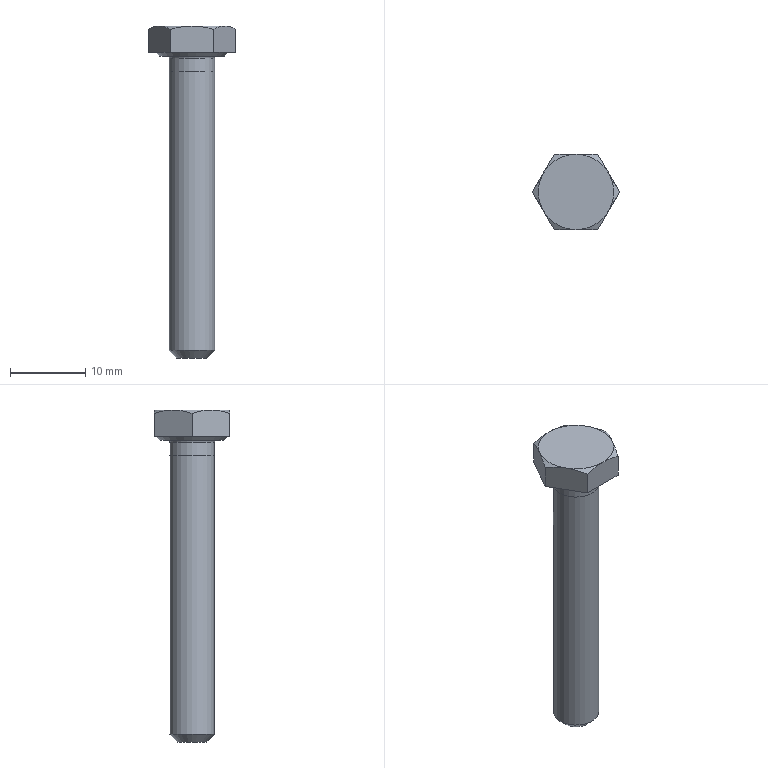Part | NX | features BREP 1, DATUM_CSYS 1 | 1 solid | 21 faces | box 11.547 x 10 x 44 mm | volume 1457 mm3 | plane 10 | cone 8 | cylinder 2 | torus 1 | commonest cylinder face diameters 6 x2
STEP:
#1=CARTESIAN_POINT('',(4.33,2.5,4.));
#2=VERTEX_POINT('',#1);
#3=CARTESIAN_POINT('',(4.33,-2.5,4.));
#4=VERTEX_POINT('',#3);
#5=CARTESIAN_POINT('',(0.,0.,4.));
#6=DIRECTION('',(0.,0.,-1.));
#7=DIRECTION('',(0.866,0.5,0.));
#8=AXIS2_PLACEMENT_3D('',#5,#6,#7);
#9=CIRCLE('',#8,5.);
#10=EDGE_CURVE('',#2,#4,#9,.T.);
#11=ORIENTED_EDGE('',*,*,#10,.F.);
#12=CARTESIAN_POINT('',(0.,5.,4.));
#13=VERTEX_POINT('',#12);
#14=CARTESIAN_POINT('',(0.,0.,4.));
#15=DIRECTION('',(0.,0.,1.));
#16=DIRECTION('',(0.866,0.5,0.));
#17=AXIS2_PLACEMENT_3D('',#14,#15,#16);
#18=CIRCLE('',#17,5.);
#19=EDGE_CURVE('',#2,#13,#18,.T.);
#20=ORIENTED_EDGE('',*,*,#19,.T.);
#21=CARTESIAN_POINT('',(-4.33,2.5,4.));
#22=VERTEX_POINT('',#21);
#23=CARTESIAN_POINT('',(0.,0.,4.));
#24=DIRECTION('',(0.,0.,1.));
#25=DIRECTION('',(0.,1.,0.));
#26=AXIS2_PLACEMENT_3D('',#23,#24,#25);
#27=CIRCLE('',#26,5.);
#28=EDGE_CURVE('',#13,#22,#27,.T.);
#29=ORIENTED_EDGE('',*,*,#28,.T.);
#30=CARTESIAN_POINT('',(-4.33,-2.5,4.));
#31=VERTEX_POINT('',#30);
#32=CARTESIAN_POINT('',(0.,0.,4.));
#33=DIRECTION('',(0.,0.,1.));
#34=DIRECTION('',(-0.866,0.5,0.));
#35=AXIS2_PLACEMENT_3D('',#32,#33,#34);
#36=CIRCLE('',#35,5.);
#37=EDGE_CURVE('',#22,#31,#36,.T.);
#38=ORIENTED_EDGE('',*,*,#37,.T.);
#39=CARTESIAN_POINT('',(0.,-5.,4.));
#40=VERTEX_POINT('',#39);
#41=CARTESIAN_POINT('',(0.,0.,4.));
#42=DIRECTION('',(0.,0.,1.));
#43=DIRECTION('',(-0.866,-0.5,0.));
#44=AXIS2_PLACEMENT_3D('',#41,#42,#43);
#45=CIRCLE('',#44,5.);
#46=EDGE_CURVE('',#31,#40,#45,.T.);
#47=ORIENTED_EDGE('',*,*,#46,.T.);
#48=CARTESIAN_POINT('',(0.,0.,4.));
#49=DIRECTION('',(0.,0.,1.));
#50=DIRECTION('',(0.,-1.,0.));
#51=AXIS2_PLACEMENT_3D('',#48,#49,#50);
#52=CIRCLE('',#51,5.);
#53=EDGE_CURVE('',#40,#4,#52,.T.);
#54=ORIENTED_EDGE('',*,*,#53,.T.);
#55=EDGE_LOOP('',(#11,#20,#29,#38,#47,#54));
#56=FACE_BOUND('',#55,.T.);
#57=CARTESIAN_POINT('',(0.,0.7735,4.));
#58=DIRECTION('',(0.,0.,1.));
#59=DIRECTION('',(-1.,0.,0.));
#60=AXIS2_PLACEMENT_3D('',#57,#58,#59);
#61=PLANE('',#60);
#62=ADVANCED_FACE('',(#56),#61,.T.);
#63=CARTESIAN_POINT('',(5.774,0.,0.5));
#64=VERTEX_POINT('',#63);
#65=CARTESIAN_POINT('',(2.887,5.,0.5));
#66=VERTEX_POINT('',#65);
#67=CARTESIAN_POINT('',(5.774,0.,0.5));
#68=DIRECTION('',(-0.5,0.866,0.));
#69=VECTOR('',#68,1000.);
#70=LINE('',#67,#69);
#71=EDGE_CURVE('',#64,#66,#70,.T.);
#72=ORIENTED_EDGE('',*,*,#71,.T.);
#73=CARTESIAN_POINT('',(2.887,5.,3.553));
#74=VERTEX_POINT('',#73);
#75=CARTESIAN_POINT('',(2.887,5.,0.5));
#76=DIRECTION('',(0.,0.,1.));
#77=VECTOR('',#76,1000.);
#78=LINE('',#75,#77);
#79=EDGE_CURVE('',#66,#74,#78,.T.);
#80=ORIENTED_EDGE('',*,*,#79,.T.);
#81=CARTESIAN_POINT('',(4.33,2.5,4.));
#82=CARTESIAN_POINT('',(3.66,3.66,4.));
#83=CARTESIAN_POINT('',(2.887,5.,3.553));
#84=(BOUNDED_CURVE()B_SPLINE_CURVE(2,(#81,#82,#83),.UNSPECIFIED.,.F.,.F.)B_SPLINE_CURVE_WITH_KNOTS((3,3),(0.,1.),.PIECEWISE_BEZIER_KNOTS.)CURVE()GEOMETRIC_REPRESENTATION_ITEM()RATIONAL_B_SPLINE_CURVE((1.544,1.544,1.434))REPRESENTATION_ITEM(''));
#85=EDGE_CURVE('',#2,#74,#84,.T.);
#86=ORIENTED_EDGE('',*,*,#85,.F.);
#87=CARTESIAN_POINT('',(5.774,0.,3.553));
#88=VERTEX_POINT('',#87);
#89=CARTESIAN_POINT('',(5.774,0.,3.553));
#90=CARTESIAN_POINT('',(5.,1.34,4.));
#91=CARTESIAN_POINT('',(4.33,2.5,4.));
#92=(BOUNDED_CURVE()B_SPLINE_CURVE(2,(#89,#90,#91),.UNSPECIFIED.,.F.,.F.)B_SPLINE_CURVE_WITH_KNOTS((3,3),(0.,1.),.PIECEWISE_BEZIER_KNOTS.)CURVE()GEOMETRIC_REPRESENTATION_ITEM()RATIONAL_B_SPLINE_CURVE((1.434,1.544,1.544))REPRESENTATION_ITEM(''));
#93=EDGE_CURVE('',#88,#2,#92,.T.);
#94=ORIENTED_EDGE('',*,*,#93,.F.);
#95=CARTESIAN_POINT('',(5.774,0.,0.5));
#96=DIRECTION('',(0.,0.,1.));
#97=VECTOR('',#96,1000.);
#98=LINE('',#95,#97);
#99=EDGE_CURVE('',#64,#88,#98,.T.);
#100=ORIENTED_EDGE('',*,*,#99,.F.);
#101=EDGE_LOOP('',(#72,#80,#86,#94,#100));
#102=FACE_BOUND('',#101,.T.);
#103=CARTESIAN_POINT('',(4.33,2.5,2.25));
#104=DIRECTION('',(0.866,0.5,0.));
#105=DIRECTION('',(0.5,-0.866,0.));
#106=AXIS2_PLACEMENT_3D('',#103,#104,#105);
#107=PLANE('',#106);
#108=ADVANCED_FACE('',(#102),#107,.T.);
#109=CARTESIAN_POINT('',(-2.887,5.,0.5));
#110=VERTEX_POINT('',#109);
#111=CARTESIAN_POINT('',(2.887,5.,0.5));
#112=DIRECTION('',(-1.,0.,0.));
#113=VECTOR('',#112,1000.);
#114=LINE('',#111,#113);
#115=EDGE_CURVE('',#66,#110,#114,.T.);
#116=ORIENTED_EDGE('',*,*,#115,.T.);
#117=CARTESIAN_POINT('',(-2.887,5.,3.553));
#118=VERTEX_POINT('',#117);
#119=CARTESIAN_POINT('',(-2.887,5.,0.5));
#120=DIRECTION('',(0.,0.,1.));
#121=VECTOR('',#120,1000.);
#122=LINE('',#119,#121);
#123=EDGE_CURVE('',#110,#118,#122,.T.);
#124=ORIENTED_EDGE('',*,*,#123,.T.);
#125=CARTESIAN_POINT('',(0.,5.,4.));
#126=CARTESIAN_POINT('',(-1.34,5.,4.));
#127=CARTESIAN_POINT('',(-2.887,5.,3.553));
#128=(BOUNDED_CURVE()B_SPLINE_CURVE(2,(#125,#126,#127),.UNSPECIFIED.,.F.,.F.)B_SPLINE_CURVE_WITH_KNOTS((3,3),(0.,1.),.PIECEWISE_BEZIER_KNOTS.)CURVE()GEOMETRIC_REPRESENTATION_ITEM()RATIONAL_B_SPLINE_CURVE((1.544,1.544,1.434))REPRESENTATION_ITEM(''));
#129=EDGE_CURVE('',#13,#118,#128,.T.);
#130=ORIENTED_EDGE('',*,*,#129,.F.);
#131=CARTESIAN_POINT('',(2.887,5.,3.553));
#132=CARTESIAN_POINT('',(1.34,5.,4.));
#133=CARTESIAN_POINT('',(0.,5.,4.));
#134=(BOUNDED_CURVE()B_SPLINE_CURVE(2,(#131,#132,#133),.UNSPECIFIED.,.F.,.F.)B_SPLINE_CURVE_WITH_KNOTS((3,3),(0.,1.),.PIECEWISE_BEZIER_KNOTS.)CURVE()GEOMETRIC_REPRESENTATION_ITEM()RATIONAL_B_SPLINE_CURVE((1.434,1.544,1.544))REPRESENTATION_ITEM(''));
#135=EDGE_CURVE('',#74,#13,#134,.T.);
#136=ORIENTED_EDGE('',*,*,#135,.F.);
#137=ORIENTED_EDGE('',*,*,#79,.F.);
#138=EDGE_LOOP('',(#116,#124,#130,#136,#137));
#139=FACE_BOUND('',#138,.T.);
#140=CARTESIAN_POINT('',(0.,5.,2.25));
#141=DIRECTION('',(0.,1.,0.));
#142=DIRECTION('',(1.,0.,0.));
#143=AXIS2_PLACEMENT_3D('',#140,#141,#142);
#144=PLANE('',#143);
#145=ADVANCED_FACE('',(#139),#144,.T.);
#146=CARTESIAN_POINT('',(-5.774,0.,0.5));
#147=VERTEX_POINT('',#146);
#148=CARTESIAN_POINT('',(-2.887,5.,0.5));
#149=DIRECTION('',(-0.5,-0.866,0.));
#150=VECTOR('',#149,1000.);
#151=LINE('',#148,#150);
#152=EDGE_CURVE('',#110,#147,#151,.T.);
#153=ORIENTED_EDGE('',*,*,#152,.T.);
#154=CARTESIAN_POINT('',(-5.774,0.,3.553));
#155=VERTEX_POINT('',#154);
#156=CARTESIAN_POINT('',(-5.774,0.,0.5));
#157=DIRECTION('',(0.,0.,1.));
#158=VECTOR('',#157,1000.);
#159=LINE('',#156,#158);
#160=EDGE_CURVE('',#147,#155,#159,.T.);
#161=ORIENTED_EDGE('',*,*,#160,.T.);
#162=CARTESIAN_POINT('',(-4.33,2.5,4.));
#163=CARTESIAN_POINT('',(-5.,1.34,4.));
#164=CARTESIAN_POINT('',(-5.774,0.,3.553));
#165=(BOUNDED_CURVE()B_SPLINE_CURVE(2,(#162,#163,#164),.UNSPECIFIED.,.F.,.F.)B_SPLINE_CURVE_WITH_KNOTS((3,3),(0.,1.),.PIECEWISE_BEZIER_KNOTS.)CURVE()GEOMETRIC_REPRESENTATION_ITEM()RATIONAL_B_SPLINE_CURVE((1.544,1.544,1.434))REPRESENTATION_ITEM(''));
#166=EDGE_CURVE('',#22,#155,#165,.T.);
#167=ORIENTED_EDGE('',*,*,#166,.F.);
#168=CARTESIAN_POINT('',(-2.887,5.,3.553));
#169=CARTESIAN_POINT('',(-3.66,3.66,4.));
#170=CARTESIAN_POINT('',(-4.33,2.5,4.));
#171=(BOUNDED_CURVE()B_SPLINE_CURVE(2,(#168,#169,#170),.UNSPECIFIED.,.F.,.F.)B_SPLINE_CURVE_WITH_KNOTS((3,3),(0.,1.),.PIECEWISE_BEZIER_KNOTS.)CURVE()GEOMETRIC_REPRESENTATION_ITEM()RATIONAL_B_SPLINE_CURVE((1.434,1.544,1.544))REPRESENTATION_ITEM(''));
#172=EDGE_CURVE('',#118,#22,#171,.T.);
#173=ORIENTED_EDGE('',*,*,#172,.F.);
#174=ORIENTED_EDGE('',*,*,#123,.F.);
#175=EDGE_LOOP('',(#153,#161,#167,#173,#174));
#176=FACE_BOUND('',#175,.T.);
#177=CARTESIAN_POINT('',(-4.33,2.5,2.25));
#178=DIRECTION('',(-0.866,0.5,0.));
#179=DIRECTION('',(0.5,0.866,0.));
#180=AXIS2_PLACEMENT_3D('',#177,#178,#179);
#181=PLANE('',#180);
#182=ADVANCED_FACE('',(#176),#181,.T.);
#183=CARTESIAN_POINT('',(-2.887,-5.,0.5));
#184=VERTEX_POINT('',#183);
#185=CARTESIAN_POINT('',(-5.774,0.,0.5));
#186=DIRECTION('',(0.5,-0.866,0.));
#187=VECTOR('',#186,1000.);
#188=LINE('',#185,#187);
#189=EDGE_CURVE('',#147,#184,#188,.T.);
#190=ORIENTED_EDGE('',*,*,#189,.T.);
#191=CARTESIAN_POINT('',(-2.887,-5.,3.553));
#192=VERTEX_POINT('',#191);
#193=CARTESIAN_POINT('',(-2.887,-5.,0.5));
#194=DIRECTION('',(0.,0.,1.));
#195=VECTOR('',#194,1000.);
#196=LINE('',#193,#195);
#197=EDGE_CURVE('',#184,#192,#196,.T.);
#198=ORIENTED_EDGE('',*,*,#197,.T.);
#199=CARTESIAN_POINT('',(-4.33,-2.5,4.));
#200=CARTESIAN_POINT('',(-3.66,-3.66,4.));
#201=CARTESIAN_POINT('',(-2.887,-5.,3.553));
#202=(BOUNDED_CURVE()B_SPLINE_CURVE(2,(#199,#200,#201),.UNSPECIFIED.,.F.,.F.)B_SPLINE_CURVE_WITH_KNOTS((3,3),(0.,1.),.PIECEWISE_BEZIER_KNOTS.)CURVE()GEOMETRIC_REPRESENTATION_ITEM()RATIONAL_B_SPLINE_CURVE((1.544,1.544,1.434))REPRESENTATION_ITEM(''));
#203=EDGE_CURVE('',#31,#192,#202,.T.);
#204=ORIENTED_EDGE('',*,*,#203,.F.);
#205=CARTESIAN_POINT('',(-5.774,0.,3.553));
#206=CARTESIAN_POINT('',(-5.,-1.34,4.));
#207=CARTESIAN_POINT('',(-4.33,-2.5,4.));
#208=(BOUNDED_CURVE()B_SPLINE_CURVE(2,(#205,#206,#207),.UNSPECIFIED.,.F.,.F.)B_SPLINE_CURVE_WITH_KNOTS((3,3),(0.,1.),.PIECEWISE_BEZIER_KNOTS.)CURVE()GEOMETRIC_REPRESENTATION_ITEM()RATIONAL_B_SPLINE_CURVE((1.434,1.544,1.544))REPRESENTATION_ITEM(''));
#209=EDGE_CURVE('',#155,#31,#208,.T.);
#210=ORIENTED_EDGE('',*,*,#209,.F.);
#211=ORIENTED_EDGE('',*,*,#160,.F.);
#212=EDGE_LOOP('',(#190,#198,#204,#210,#211));
#213=FACE_BOUND('',#212,.T.);
#214=CARTESIAN_POINT('',(-4.33,-2.5,2.25));
#215=DIRECTION('',(-0.866,-0.5,0.));
#216=DIRECTION('',(-0.5,0.866,0.));
#217=AXIS2_PLACEMENT_3D('',#214,#215,#216);
#218=PLANE('',#217);
#219=ADVANCED_FACE('',(#213),#218,.T.);
#220=CARTESIAN_POINT('',(2.887,-5.,0.5));
#221=VERTEX_POINT('',#220);
#222=CARTESIAN_POINT('',(-2.887,-5.,0.5));
#223=DIRECTION('',(1.,0.,0.));
#224=VECTOR('',#223,1000.);
#225=LINE('',#222,#224);
#226=EDGE_CURVE('',#184,#221,#225,.T.);
#227=ORIENTED_EDGE('',*,*,#226,.T.);
#228=CARTESIAN_POINT('',(2.887,-5.,3.553));
#229=VERTEX_POINT('',#228);
#230=CARTESIAN_POINT('',(2.887,-5.,0.5));
#231=DIRECTION('',(0.,0.,1.));
#232=VECTOR('',#231,1000.);
#233=LINE('',#230,#232);
#234=EDGE_CURVE('',#221,#229,#233,.T.);
#235=ORIENTED_EDGE('',*,*,#234,.T.);
#236=CARTESIAN_POINT('',(0.,-5.,4.));
#237=CARTESIAN_POINT('',(1.34,-5.,4.));
#238=CARTESIAN_POINT('',(2.887,-5.,3.553));
#239=(BOUNDED_CURVE()B_SPLINE_CURVE(2,(#236,#237,#238),.UNSPECIFIED.,.F.,.F.)B_SPLINE_CURVE_WITH_KNOTS((3,3),(0.,1.),.PIECEWISE_BEZIER_KNOTS.)CURVE()GEOMETRIC_REPRESENTATION_ITEM()RATIONAL_B_SPLINE_CURVE((1.544,1.544,1.434))REPRESENTATION_ITEM(''));
#240=EDGE_CURVE('',#40,#229,#239,.T.);
#241=ORIENTED_EDGE('',*,*,#240,.F.);
#242=CARTESIAN_POINT('',(-2.887,-5.,3.553));
#243=CARTESIAN_POINT('',(-1.34,-5.,4.));
#244=CARTESIAN_POINT('',(0.,-5.,4.));
#245=(BOUNDED_CURVE()B_SPLINE_CURVE(2,(#242,#243,#244),.UNSPECIFIED.,.F.,.F.)B_SPLINE_CURVE_WITH_KNOTS((3,3),(0.,1.),.PIECEWISE_BEZIER_KNOTS.)CURVE()GEOMETRIC_REPRESENTATION_ITEM()RATIONAL_B_SPLINE_CURVE((1.434,1.544,1.544))REPRESENTATION_ITEM(''));
#246=EDGE_CURVE('',#192,#40,#245,.T.);
#247=ORIENTED_EDGE('',*,*,#246,.F.);
#248=ORIENTED_EDGE('',*,*,#197,.F.);
#249=EDGE_LOOP('',(#227,#235,#241,#247,#248));
#250=FACE_BOUND('',#249,.T.);
#251=CARTESIAN_POINT('',(0.,-5.,2.25));
#252=DIRECTION('',(0.,-1.,0.));
#253=DIRECTION('',(-1.,0.,0.));
#254=AXIS2_PLACEMENT_3D('',#251,#252,#253);
#255=PLANE('',#254);
#256=ADVANCED_FACE('',(#250),#255,.T.);
#257=CARTESIAN_POINT('',(2.887,-5.,0.5));
#258=DIRECTION('',(0.5,0.866,0.));
#259=VECTOR('',#258,1000.);
#260=LINE('',#257,#259);
#261=EDGE_CURVE('',#221,#64,#260,.T.);
#262=ORIENTED_EDGE('',*,*,#261,.T.);
#263=ORIENTED_EDGE('',*,*,#99,.T.);
#264=CARTESIAN_POINT('',(4.33,-2.5,4.));
#265=CARTESIAN_POINT('',(5.,-1.34,4.));
#266=CARTESIAN_POINT('',(5.774,0.,3.553));
#267=(BOUNDED_CURVE()B_SPLINE_CURVE(2,(#264,#265,#266),.UNSPECIFIED.,.F.,.F.)B_SPLINE_CURVE_WITH_KNOTS((3,3),(0.,1.),.PIECEWISE_BEZIER_KNOTS.)CURVE()GEOMETRIC_REPRESENTATION_ITEM()RATIONAL_B_SPLINE_CURVE((1.544,1.544,1.434))REPRESENTATION_ITEM(''));
#268=EDGE_CURVE('',#4,#88,#267,.T.);
#269=ORIENTED_EDGE('',*,*,#268,.F.);
#270=CARTESIAN_POINT('',(2.887,-5.,3.553));
#271=CARTESIAN_POINT('',(3.66,-3.66,4.));
#272=CARTESIAN_POINT('',(4.33,-2.5,4.));
#273=(BOUNDED_CURVE()B_SPLINE_CURVE(2,(#270,#271,#272),.UNSPECIFIED.,.F.,.F.)B_SPLINE_CURVE_WITH_KNOTS((3,3),(0.,1.),.PIECEWISE_BEZIER_KNOTS.)CURVE()GEOMETRIC_REPRESENTATION_ITEM()RATIONAL_B_SPLINE_CURVE((1.434,1.544,1.544))REPRESENTATION_ITEM(''));
#274=EDGE_CURVE('',#229,#4,#273,.T.);
#275=ORIENTED_EDGE('',*,*,#274,.F.);
#276=ORIENTED_EDGE('',*,*,#234,.F.);
#277=EDGE_LOOP('',(#262,#263,#269,#275,#276));
#278=FACE_BOUND('',#277,.T.);
#279=CARTESIAN_POINT('',(4.33,-2.5,2.25));
#280=DIRECTION('',(0.866,-0.5,0.));
#281=DIRECTION('',(-0.5,-0.866,0.));
#282=AXIS2_PLACEMENT_3D('',#279,#280,#281);
#283=PLANE('',#282);
#284=ADVANCED_FACE('',(#278),#283,.T.);
#285=ORIENTED_EDGE('',*,*,#261,.F.);
#286=ORIENTED_EDGE('',*,*,#226,.F.);
#287=ORIENTED_EDGE('',*,*,#189,.F.);
#288=ORIENTED_EDGE('',*,*,#152,.F.);
#289=ORIENTED_EDGE('',*,*,#115,.F.);
#290=ORIENTED_EDGE('',*,*,#71,.F.);
#291=EDGE_LOOP('',(#285,#286,#287,#288,#289,#290));
#292=FACE_BOUND('',#291,.T.);
#293=CARTESIAN_POINT('',(4.77,0.,0.5));
#294=VERTEX_POINT('',#293);
#295=CARTESIAN_POINT('',(0.,0.,0.5));
#296=DIRECTION('',(0.,0.,1.));
#297=DIRECTION('',(1.,0.,0.));
#298=AXIS2_PLACEMENT_3D('',#295,#296,#297);
#299=CIRCLE('',#298,4.77);
#300=EDGE_CURVE('',#294,#294,#299,.T.);
#301=ORIENTED_EDGE('',*,*,#300,.T.);
#302=EDGE_LOOP('',(#301));
#303=FACE_BOUND('',#302,.T.);
#304=CARTESIAN_POINT('',(0.,0.7735,0.5));
#305=DIRECTION('',(0.,0.,1.));
#306=DIRECTION('',(-1.,0.,0.));
#307=AXIS2_PLACEMENT_3D('',#304,#305,#306);
#308=PLANE('',#307);
#309=ADVANCED_FACE('',(#292,#303),#308,.F.);
#310=CARTESIAN_POINT('',(4.27,0.,0.));
#311=VERTEX_POINT('',#310);
#312=CARTESIAN_POINT('',(0.,0.,0.));
#313=DIRECTION('',(0.,0.,1.));
#314=DIRECTION('',(1.,0.,0.));
#315=AXIS2_PLACEMENT_3D('',#312,#313,#314);
#316=CIRCLE('',#315,4.27);
#317=EDGE_CURVE('',#311,#311,#316,.T.);
#318=ORIENTED_EDGE('',*,*,#317,.T.);
#319=CARTESIAN_POINT('',(4.27,0.,0.));
#320=DIRECTION('',(0.7071,0.,0.7071));
#321=VECTOR('',#320,1000.);
#322=LINE('',#319,#321);
#323=EDGE_CURVE('',#311,#294,#322,.T.);
#324=ORIENTED_EDGE('',*,*,#323,.T.);
#325=ORIENTED_EDGE('',*,*,#300,.F.);
#326=ORIENTED_EDGE('',*,*,#323,.F.);
#327=EDGE_LOOP('',(#318,#324,#325,#326));
#328=FACE_BOUND('',#327,.T.);
#329=CARTESIAN_POINT('',(0.,0.,0.));
#330=DIRECTION('',(0.,0.,1.));
#331=DIRECTION('',(-1.,0.,0.));
#332=AXIS2_PLACEMENT_3D('',#329,#330,#331);
#333=CONICAL_SURFACE('',#332,4.27,0.7854);
#334=ADVANCED_FACE('',(#328),#333,.T.);
#335=ORIENTED_EDGE('',*,*,#317,.F.);
#336=EDGE_LOOP('',(#335));
#337=FACE_BOUND('',#336,.T.);
#338=CARTESIAN_POINT('',(3.25,0.,0.));
#339=VERTEX_POINT('',#338);
#340=CARTESIAN_POINT('',(0.,0.,0.));
#341=DIRECTION('',(0.,0.,1.));
#342=DIRECTION('',(1.,0.,0.));
#343=AXIS2_PLACEMENT_3D('',#340,#341,#342);
#344=CIRCLE('',#343,3.25);
#345=EDGE_CURVE('',#339,#339,#344,.T.);
#346=ORIENTED_EDGE('',*,*,#345,.T.);
#347=EDGE_LOOP('',(#346));
#348=FACE_BOUND('',#347,.T.);
#349=CARTESIAN_POINT('',(0.,0.,0.));
#350=DIRECTION('',(0.,0.,1.));
#351=DIRECTION('',(-1.,0.,0.));
#352=AXIS2_PLACEMENT_3D('',#349,#350,#351);
#353=PLANE('',#352);
#354=ADVANCED_FACE('',(#337,#348),#353,.F.);
#355=CARTESIAN_POINT('',(3.,0.,-0.25));
#356=VERTEX_POINT('',#355);
#357=CARTESIAN_POINT('',(0.,0.,-0.25));
#358=DIRECTION('',(0.,0.,1.));
#359=DIRECTION('',(1.,0.,0.));
#360=AXIS2_PLACEMENT_3D('',#357,#358,#359);
#361=CIRCLE('',#360,3.);
#362=EDGE_CURVE('',#356,#356,#361,.T.);
#363=ORIENTED_EDGE('',*,*,#362,.T.);
#364=CARTESIAN_POINT('',(3.25,0.,-0.25));
#365=DIRECTION('',(0.,1.,0.));
#366=DIRECTION('',(-1.,0.,0.));
#367=AXIS2_PLACEMENT_3D('',#364,#365,#366);
#368=CIRCLE('',#367,0.25);
#369=EDGE_CURVE('',#356,#339,#368,.T.);
#370=ORIENTED_EDGE('',*,*,#369,.T.);
#371=ORIENTED_EDGE('',*,*,#345,.F.);
#372=ORIENTED_EDGE('',*,*,#369,.F.);
#373=EDGE_LOOP('',(#363,#370,#371,#372));
#374=FACE_BOUND('',#373,.T.);
#375=CARTESIAN_POINT('',(0.,0.,-0.25));
#376=DIRECTION('',(0.,0.,-1.));
#377=DIRECTION('',(-1.,0.,0.));
#378=AXIS2_PLACEMENT_3D('',#375,#376,#377);
#379=TOROIDAL_SURFACE('',#378,3.25,0.25);
#380=ADVANCED_FACE('',(#374),#379,.F.);
#381=CARTESIAN_POINT('',(3.,0.,-2.));
#382=VERTEX_POINT('',#381);
#383=CARTESIAN_POINT('',(0.,0.,-2.));
#384=DIRECTION('',(0.,0.,1.));
#385=DIRECTION('',(1.,0.,0.));
#386=AXIS2_PLACEMENT_3D('',#383,#384,#385);
#387=CIRCLE('',#386,3.);
#388=EDGE_CURVE('',#382,#382,#387,.T.);
#389=ORIENTED_EDGE('',*,*,#388,.T.);
#390=CARTESIAN_POINT('',(3.,0.,-2.));
#391=DIRECTION('',(0.,0.,1.));
#392=VECTOR('',#391,1000.);
#393=LINE('',#390,#392);
#394=EDGE_CURVE('',#382,#356,#393,.T.);
#395=ORIENTED_EDGE('',*,*,#394,.T.);
#396=ORIENTED_EDGE('',*,*,#362,.F.);
#397=ORIENTED_EDGE('',*,*,#394,.F.);
#398=EDGE_LOOP('',(#389,#395,#396,#397));
#399=FACE_BOUND('',#398,.T.);
#400=CARTESIAN_POINT('',(0.,0.,-2.));
#401=DIRECTION('',(0.,0.,1.));
#402=DIRECTION('',(-1.,0.,0.));
#403=AXIS2_PLACEMENT_3D('',#400,#401,#402);
#404=CYLINDRICAL_SURFACE('',#403,3.);
#405=ADVANCED_FACE('',(#399),#404,.T.);
#406=CARTESIAN_POINT('',(3.,0.,-39.));
#407=VERTEX_POINT('',#406);
#408=CARTESIAN_POINT('',(0.,0.,-39.));
#409=DIRECTION('',(0.,0.,1.));
#410=DIRECTION('',(1.,0.,0.));
#411=AXIS2_PLACEMENT_3D('',#408,#409,#410);
#412=CIRCLE('',#411,3.);
#413=EDGE_CURVE('',#407,#407,#412,.T.);
#414=ORIENTED_EDGE('',*,*,#413,.T.);
#415=CARTESIAN_POINT('',(3.,0.,-39.));
#416=DIRECTION('',(0.,0.,1.));
#417=VECTOR('',#416,1000.);
#418=LINE('',#415,#417);
#419=EDGE_CURVE('',#407,#382,#418,.T.);
#420=ORIENTED_EDGE('',*,*,#419,.T.);
#421=ORIENTED_EDGE('',*,*,#388,.F.);
#422=ORIENTED_EDGE('',*,*,#419,.F.);
#423=EDGE_LOOP('',(#414,#420,#421,#422));
#424=FACE_BOUND('',#423,.T.);
#425=CARTESIAN_POINT('',(0.,0.,-39.));
#426=DIRECTION('',(0.,0.,1.));
#427=DIRECTION('',(-1.,0.,0.));
#428=AXIS2_PLACEMENT_3D('',#425,#426,#427);
#429=CYLINDRICAL_SURFACE('',#428,3.);
#430=ADVANCED_FACE('',(#424),#429,.T.);
#431=CARTESIAN_POINT('',(2.,0.,-40.));
#432=VERTEX_POINT('',#431);
#433=CARTESIAN_POINT('',(0.,0.,-40.));
#434=DIRECTION('',(0.,0.,1.));
#435=DIRECTION('',(1.,0.,0.));
#436=AXIS2_PLACEMENT_3D('',#433,#434,#435);
#437=CIRCLE('',#436,2.);
#438=EDGE_CURVE('',#432,#432,#437,.T.);
#439=ORIENTED_EDGE('',*,*,#438,.T.);
#440=CARTESIAN_POINT('',(2.,0.,-40.));
#441=DIRECTION('',(0.7071,0.,0.7071));
#442=VECTOR('',#441,1000.);
#443=LINE('',#440,#442);
#444=EDGE_CURVE('',#432,#407,#443,.T.);
#445=ORIENTED_EDGE('',*,*,#444,.T.);
#446=ORIENTED_EDGE('',*,*,#413,.F.);
#447=ORIENTED_EDGE('',*,*,#444,.F.);
#448=EDGE_LOOP('',(#439,#445,#446,#447));
#449=FACE_BOUND('',#448,.T.);
#450=CARTESIAN_POINT('',(0.,0.,-40.));
#451=DIRECTION('',(0.,0.,1.));
#452=DIRECTION('',(-1.,0.,0.));
#453=AXIS2_PLACEMENT_3D('',#450,#451,#452);
#454=CONICAL_SURFACE('',#453,2.,0.7854);
#455=ADVANCED_FACE('',(#449),#454,.T.);
#456=ORIENTED_EDGE('',*,*,#438,.F.);
#457=EDGE_LOOP('',(#456));
#458=FACE_BOUND('',#457,.T.);
#459=CARTESIAN_POINT('',(0.,0.,-40.));
#460=DIRECTION('',(0.,0.,1.));
#461=DIRECTION('',(-1.,0.,0.));
#462=AXIS2_PLACEMENT_3D('',#459,#460,#461);
#463=PLANE('',#462);
#464=ADVANCED_FACE('',(#458),#463,.F.);
#465=ORIENTED_EDGE('',*,*,#19,.F.);
#466=ORIENTED_EDGE('',*,*,#85,.T.);
#467=ORIENTED_EDGE('',*,*,#135,.T.);
#468=EDGE_LOOP('',(#465,#466,#467));
#469=FACE_BOUND('',#468,.T.);
#470=CARTESIAN_POINT('',(0.,0.,4.));
#471=DIRECTION('',(0.,0.,-1.));
#472=DIRECTION('',(-0.9128,-0.4084,0.));
#473=AXIS2_PLACEMENT_3D('',#470,#471,#472);
#474=CONICAL_SURFACE('',#473,5.,1.047);
#475=ADVANCED_FACE('',(#469),#474,.T.);
#476=ORIENTED_EDGE('',*,*,#93,.T.);
#477=ORIENTED_EDGE('',*,*,#10,.T.);
#478=ORIENTED_EDGE('',*,*,#268,.T.);
#479=EDGE_LOOP('',(#476,#477,#478));
#480=FACE_BOUND('',#479,.T.);
#481=CARTESIAN_POINT('',(0.,0.,4.));
#482=DIRECTION('',(0.,0.,-1.));
#483=DIRECTION('',(-0.866,0.5,0.));
#484=AXIS2_PLACEMENT_3D('',#481,#482,#483);
#485=CONICAL_SURFACE('',#484,5.,1.047);
#486=ADVANCED_FACE('',(#480),#485,.T.);
#487=ORIENTED_EDGE('',*,*,#28,.F.);
#488=ORIENTED_EDGE('',*,*,#129,.T.);
#489=ORIENTED_EDGE('',*,*,#172,.T.);
#490=EDGE_LOOP('',(#487,#488,#489));
#491=FACE_BOUND('',#490,.T.);
#492=CARTESIAN_POINT('',(0.,0.,4.));
#493=DIRECTION('',(0.,0.,-1.));
#494=DIRECTION('',(-0.9128,-0.4084,0.));
#495=AXIS2_PLACEMENT_3D('',#492,#493,#494);
#496=CONICAL_SURFACE('',#495,5.,1.047);
#497=ADVANCED_FACE('',(#491),#496,.T.);
#498=ORIENTED_EDGE('',*,*,#37,.F.);
#499=ORIENTED_EDGE('',*,*,#166,.T.);
#500=ORIENTED_EDGE('',*,*,#209,.T.);
#501=EDGE_LOOP('',(#498,#499,#500));
#502=FACE_BOUND('',#501,.T.);
#503=CARTESIAN_POINT('',(0.,0.,4.));
#504=DIRECTION('',(0.,0.,-1.));
#505=DIRECTION('',(-0.9128,-0.4084,0.));
#506=AXIS2_PLACEMENT_3D('',#503,#504,#505);
#507=CONICAL_SURFACE('',#506,5.,1.047);
#508=ADVANCED_FACE('',(#502),#507,.T.);
#509=ORIENTED_EDGE('',*,*,#46,.F.);
#510=ORIENTED_EDGE('',*,*,#203,.T.);
#511=ORIENTED_EDGE('',*,*,#246,.T.);
#512=EDGE_LOOP('',(#509,#510,#511));
#513=FACE_BOUND('',#512,.T.);
#514=CARTESIAN_POINT('',(0.,0.,4.));
#515=DIRECTION('',(0.,0.,-1.));
#516=DIRECTION('',(-0.9128,-0.4084,0.));
#517=AXIS2_PLACEMENT_3D('',#514,#515,#516);
#518=CONICAL_SURFACE('',#517,5.,1.047);
#519=ADVANCED_FACE('',(#513),#518,.T.);
#520=ORIENTED_EDGE('',*,*,#53,.F.);
#521=ORIENTED_EDGE('',*,*,#240,.T.);
#522=ORIENTED_EDGE('',*,*,#274,.T.);
#523=EDGE_LOOP('',(#520,#521,#522));
#524=FACE_BOUND('',#523,.T.);
#525=CARTESIAN_POINT('',(0.,0.,4.));
#526=DIRECTION('',(0.,0.,-1.));
#527=DIRECTION('',(-0.9128,-0.4084,0.));
#528=AXIS2_PLACEMENT_3D('',#525,#526,#527);
#529=CONICAL_SURFACE('',#528,5.,1.047);
#530=ADVANCED_FACE('',(#524),#529,.T.);
#531=CLOSED_SHELL('',(#62,#108,#145,#182,#219,#256,#284,#309,#334,#354,#380,#405,#430,#455,#464,#475,#486,#497,#508,#519,#530));
#532=MANIFOLD_SOLID_BREP('',#531);
#533=(LENGTH_UNIT()NAMED_UNIT(*)SI_UNIT(.MILLI.,.METRE.));
#534=UNCERTAINTY_MEASURE_WITH_UNIT(LENGTH_MEASURE(0.00001),#533,'','');
#535=(NAMED_UNIT(*)PLANE_ANGLE_UNIT()SI_UNIT($,.RADIAN.));
#536=(NAMED_UNIT(*)SI_UNIT($,.STERADIAN.)SOLID_ANGLE_UNIT());
#537=(GEOMETRIC_REPRESENTATION_CONTEXT(3)GLOBAL_UNCERTAINTY_ASSIGNED_CONTEXT((#534))GLOBAL_UNIT_ASSIGNED_CONTEXT((#533,#535,#536))REPRESENTATION_CONTEXT('',''));
#538=ADVANCED_BREP_SHAPE_REPRESENTATION('',(#532),#537);